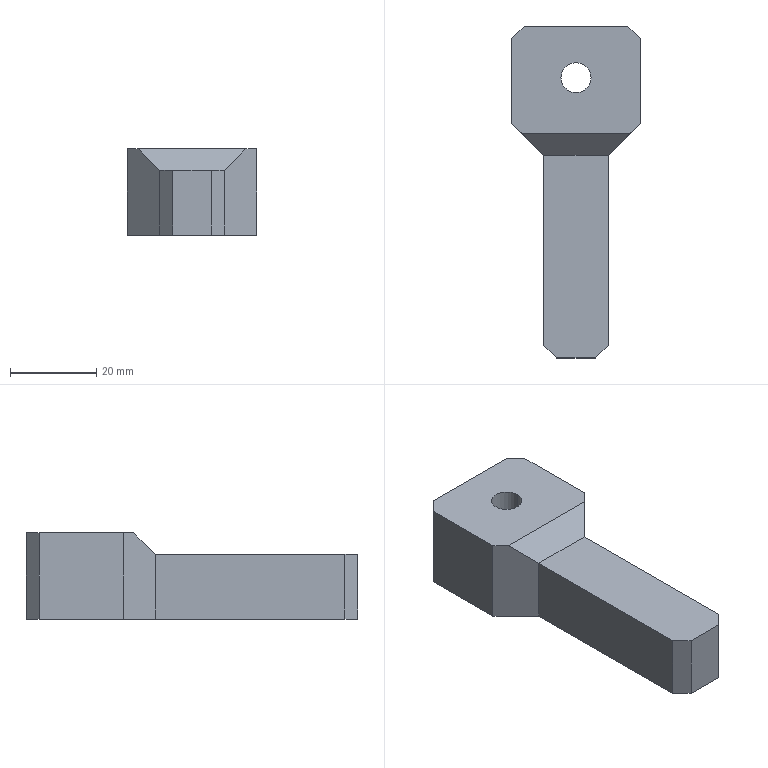Part | SolidWorks | features Chamfer 4, ICE 3, Cut 1, Extrusion 1 | 1 solid | 21 faces | box 30 x 77 x 20 mm | volume 24023 mm3 | plane 17 | cylinder 4 | commonest cylinder face diameters 7 x2 16 x2
STEP:
#1=CARTESIAN_POINT('',(-1.66,24.408,20.));
#2=VERTEX_POINT('',#1);
#3=CARTESIAN_POINT('',(-8.66,24.408,20.));
#4=VERTEX_POINT('',#3);
#5=CARTESIAN_POINT('',(-5.16,24.408,20.));
#6=DIRECTION('',(0.,0.,-1.));
#7=DIRECTION('',(-1.,0.,0.));
#8=AXIS2_PLACEMENT_3D('',#5,#6,#7);
#9=CIRCLE('',#8,3.5);
#10=EDGE_CURVE('',#2,#4,#9,.T.);
#11=ORIENTED_EDGE('',*,*,#10,.F.);
#12=CARTESIAN_POINT('',(-1.66,24.408,13.));
#13=VERTEX_POINT('',#12);
#14=CARTESIAN_POINT('',(-1.66,24.408,20.));
#15=DIRECTION('',(0.,0.,-1.));
#16=VECTOR('',#15,1000.);
#17=LINE('',#14,#16);
#18=EDGE_CURVE('',#2,#13,#17,.T.);
#19=ORIENTED_EDGE('',*,*,#18,.T.);
#20=CARTESIAN_POINT('',(-8.66,24.408,13.));
#21=VERTEX_POINT('',#20);
#22=CARTESIAN_POINT('',(-5.16,24.408,13.));
#23=DIRECTION('',(0.,0.,-1.));
#24=DIRECTION('',(-1.,0.,0.));
#25=AXIS2_PLACEMENT_3D('',#22,#23,#24);
#26=CIRCLE('',#25,3.5);
#27=EDGE_CURVE('',#13,#21,#26,.T.);
#28=ORIENTED_EDGE('',*,*,#27,.T.);
#29=CARTESIAN_POINT('',(-8.66,24.408,20.));
#30=DIRECTION('',(0.,0.,-1.));
#31=VECTOR('',#30,1000.);
#32=LINE('',#29,#31);
#33=EDGE_CURVE('',#4,#21,#32,.T.);
#34=ORIENTED_EDGE('',*,*,#33,.F.);
#35=EDGE_LOOP('',(#11,#19,#28,#34));
#36=FACE_OUTER_BOUND('',#35,.T.);
#37=CARTESIAN_POINT('',(-5.16,24.408,20.));
#38=DIRECTION('',(0.,0.,-1.));
#39=DIRECTION('',(-1.,0.,0.));
#40=AXIS2_PLACEMENT_3D('',#37,#38,#39);
#41=CYLINDRICAL_SURFACE('',#40,3.5);
#42=ADVANCED_FACE('',(#36),#41,.F.);
#43=CARTESIAN_POINT('',(2.84,24.408,13.));
#44=VERTEX_POINT('',#43);
#45=CARTESIAN_POINT('',(-13.16,24.408,13.));
#46=VERTEX_POINT('',#45);
#47=CARTESIAN_POINT('',(-5.16,24.408,13.));
#48=DIRECTION('',(0.,0.,-1.));
#49=DIRECTION('',(-1.,0.,0.));
#50=AXIS2_PLACEMENT_3D('',#47,#48,#49);
#51=CIRCLE('',#50,8.);
#52=EDGE_CURVE('',#44,#46,#51,.T.);
#53=ORIENTED_EDGE('',*,*,#52,.F.);
#54=CARTESIAN_POINT('',(2.84,24.408,0.));
#55=VERTEX_POINT('',#54);
#56=CARTESIAN_POINT('',(2.84,24.408,13.));
#57=DIRECTION('',(0.,0.,-1.));
#58=VECTOR('',#57,1000.);
#59=LINE('',#56,#58);
#60=EDGE_CURVE('',#44,#55,#59,.T.);
#61=ORIENTED_EDGE('',*,*,#60,.T.);
#62=CARTESIAN_POINT('',(-13.16,24.408,0.));
#63=VERTEX_POINT('',#62);
#64=CARTESIAN_POINT('',(-5.16,24.408,0.));
#65=DIRECTION('',(0.,0.,-1.));
#66=DIRECTION('',(-1.,0.,0.));
#67=AXIS2_PLACEMENT_3D('',#64,#65,#66);
#68=CIRCLE('',#67,8.);
#69=EDGE_CURVE('',#55,#63,#68,.T.);
#70=ORIENTED_EDGE('',*,*,#69,.T.);
#71=CARTESIAN_POINT('',(-13.16,24.408,13.));
#72=DIRECTION('',(0.,0.,-1.));
#73=VECTOR('',#72,1000.);
#74=LINE('',#71,#73);
#75=EDGE_CURVE('',#46,#63,#74,.T.);
#76=ORIENTED_EDGE('',*,*,#75,.F.);
#77=EDGE_LOOP('',(#53,#61,#70,#76));
#78=FACE_OUTER_BOUND('',#77,.T.);
#79=CARTESIAN_POINT('',(-5.16,24.408,13.));
#80=DIRECTION('',(0.,0.,-1.));
#81=DIRECTION('',(-1.,0.,0.));
#82=AXIS2_PLACEMENT_3D('',#79,#80,#81);
#83=CYLINDRICAL_SURFACE('',#82,8.);
#84=ADVANCED_FACE('',(#78),#83,.F.);
#85=CARTESIAN_POINT('',(-20.16,33.408,20.));
#86=VERTEX_POINT('',#85);
#87=CARTESIAN_POINT('',(-20.16,13.908,20.));
#88=VERTEX_POINT('',#87);
#89=CARTESIAN_POINT('',(-20.16,36.408,20.));
#90=DIRECTION('',(0.,-1.,0.));
#91=VECTOR('',#90,1000.);
#92=LINE('',#89,#91);
#93=EDGE_CURVE('',#86,#88,#92,.T.);
#94=ORIENTED_EDGE('',*,*,#93,.F.);
#95=CARTESIAN_POINT('',(-20.16,33.408,0.));
#96=VERTEX_POINT('',#95);
#97=CARTESIAN_POINT('',(-20.16,33.408,20.));
#98=DIRECTION('',(0.,0.,-1.));
#99=VECTOR('',#98,1000.);
#100=LINE('',#97,#99);
#101=EDGE_CURVE('',#86,#96,#100,.T.);
#102=ORIENTED_EDGE('',*,*,#101,.T.);
#103=CARTESIAN_POINT('',(-20.16,13.908,0.));
#104=VERTEX_POINT('',#103);
#105=CARTESIAN_POINT('',(-20.16,36.408,0.));
#106=DIRECTION('',(0.,-1.,0.));
#107=VECTOR('',#106,1000.);
#108=LINE('',#105,#107);
#109=EDGE_CURVE('',#96,#104,#108,.T.);
#110=ORIENTED_EDGE('',*,*,#109,.T.);
#111=CARTESIAN_POINT('',(-20.16,13.908,20.));
#112=DIRECTION('',(0.,0.,1.));
#113=VECTOR('',#112,1000.);
#114=LINE('',#111,#113);
#115=EDGE_CURVE('',#104,#88,#114,.T.);
#116=ORIENTED_EDGE('',*,*,#115,.T.);
#117=EDGE_LOOP('',(#94,#102,#110,#116));
#118=FACE_OUTER_BOUND('',#117,.T.);
#119=CARTESIAN_POINT('',(-20.16,36.408,20.));
#120=DIRECTION('',(1.,0.,0.));
#121=DIRECTION('',(0.,1.,0.));
#122=AXIS2_PLACEMENT_3D('',#119,#120,#121);
#123=PLANE('',#122);
#124=ADVANCED_FACE('',(#118),#123,.F.);
#125=CARTESIAN_POINT('',(-0.6603,-40.592,0.));
#126=VERTEX_POINT('',#125);
#127=CARTESIAN_POINT('',(-0.6603,-40.592,15.));
#128=VERTEX_POINT('',#127);
#129=CARTESIAN_POINT('',(-0.6603,-40.592,20.));
#130=DIRECTION('',(0.,0.,1.));
#131=VECTOR('',#130,1000.);
#132=LINE('',#129,#131);
#133=EDGE_CURVE('',#126,#128,#132,.T.);
#134=ORIENTED_EDGE('',*,*,#133,.T.);
#135=CARTESIAN_POINT('',(-9.66,-40.592,15.));
#136=VERTEX_POINT('',#135);
#137=CARTESIAN_POINT('',(-20.16,-40.592,15.));
#138=DIRECTION('',(-1.,0.,0.));
#139=VECTOR('',#138,1000.);
#140=LINE('',#137,#139);
#141=EDGE_CURVE('',#128,#136,#140,.T.);
#142=ORIENTED_EDGE('',*,*,#141,.T.);
#143=CARTESIAN_POINT('',(-9.66,-40.592,0.));
#144=VERTEX_POINT('',#143);
#145=CARTESIAN_POINT('',(-9.66,-40.592,20.));
#146=DIRECTION('',(0.,0.,-1.));
#147=VECTOR('',#146,1000.);
#148=LINE('',#145,#147);
#149=EDGE_CURVE('',#136,#144,#148,.T.);
#150=ORIENTED_EDGE('',*,*,#149,.T.);
#151=CARTESIAN_POINT('',(-20.16,-40.592,0.));
#152=DIRECTION('',(1.,0.,0.));
#153=VECTOR('',#152,1000.);
#154=LINE('',#151,#153);
#155=EDGE_CURVE('',#144,#126,#154,.T.);
#156=ORIENTED_EDGE('',*,*,#155,.T.);
#157=EDGE_LOOP('',(#134,#142,#150,#156));
#158=FACE_OUTER_BOUND('',#157,.T.);
#159=CARTESIAN_POINT('',(-20.16,-40.592,20.));
#160=DIRECTION('',(0.,1.,0.));
#161=DIRECTION('',(0.,0.,1.));
#162=AXIS2_PLACEMENT_3D('',#159,#160,#161);
#163=PLANE('',#162);
#164=ADVANCED_FACE('',(#158),#163,.F.);
#165=CARTESIAN_POINT('',(9.84,13.908,0.));
#166=VERTEX_POINT('',#165);
#167=CARTESIAN_POINT('',(9.84,33.408,0.));
#168=VERTEX_POINT('',#167);
#169=CARTESIAN_POINT('',(9.84,36.408,0.));
#170=DIRECTION('',(0.,1.,0.));
#171=VECTOR('',#170,1000.);
#172=LINE('',#169,#171);
#173=EDGE_CURVE('',#166,#168,#172,.T.);
#174=ORIENTED_EDGE('',*,*,#173,.T.);
#175=CARTESIAN_POINT('',(9.84,33.408,20.));
#176=VERTEX_POINT('',#175);
#177=CARTESIAN_POINT('',(9.84,33.408,20.));
#178=DIRECTION('',(0.,0.,1.));
#179=VECTOR('',#178,1000.);
#180=LINE('',#177,#179);
#181=EDGE_CURVE('',#168,#176,#180,.T.);
#182=ORIENTED_EDGE('',*,*,#181,.T.);
#183=CARTESIAN_POINT('',(9.84,13.908,20.));
#184=VERTEX_POINT('',#183);
#185=CARTESIAN_POINT('',(9.84,36.408,20.));
#186=DIRECTION('',(0.,1.,0.));
#187=VECTOR('',#186,1000.);
#188=LINE('',#185,#187);
#189=EDGE_CURVE('',#184,#176,#188,.T.);
#190=ORIENTED_EDGE('',*,*,#189,.F.);
#191=CARTESIAN_POINT('',(9.84,13.908,20.));
#192=DIRECTION('',(0.,0.,-1.));
#193=VECTOR('',#192,1000.);
#194=LINE('',#191,#193);
#195=EDGE_CURVE('',#184,#166,#194,.T.);
#196=ORIENTED_EDGE('',*,*,#195,.T.);
#197=EDGE_LOOP('',(#174,#182,#190,#196));
#198=FACE_OUTER_BOUND('',#197,.T.);
#199=CARTESIAN_POINT('',(9.84,36.408,20.));
#200=DIRECTION('',(-1.,0.,0.));
#201=DIRECTION('',(0.,-1.,0.));
#202=AXIS2_PLACEMENT_3D('',#199,#200,#201);
#203=PLANE('',#202);
#204=ADVANCED_FACE('',(#198),#203,.F.);
#205=CARTESIAN_POINT('',(6.84,36.408,20.));
#206=VERTEX_POINT('',#205);
#207=CARTESIAN_POINT('',(-17.16,36.408,20.));
#208=VERTEX_POINT('',#207);
#209=CARTESIAN_POINT('',(-20.16,36.408,20.));
#210=DIRECTION('',(-1.,0.,0.));
#211=VECTOR('',#210,1000.);
#212=LINE('',#209,#211);
#213=EDGE_CURVE('',#206,#208,#212,.T.);
#214=ORIENTED_EDGE('',*,*,#213,.F.);
#215=CARTESIAN_POINT('',(6.84,36.408,0.));
#216=VERTEX_POINT('',#215);
#217=CARTESIAN_POINT('',(6.84,36.408,20.));
#218=DIRECTION('',(0.,0.,-1.));
#219=VECTOR('',#218,1000.);
#220=LINE('',#217,#219);
#221=EDGE_CURVE('',#206,#216,#220,.T.);
#222=ORIENTED_EDGE('',*,*,#221,.T.);
#223=CARTESIAN_POINT('',(-17.16,36.408,0.));
#224=VERTEX_POINT('',#223);
#225=CARTESIAN_POINT('',(-20.16,36.408,0.));
#226=DIRECTION('',(-1.,0.,0.));
#227=VECTOR('',#226,1000.);
#228=LINE('',#225,#227);
#229=EDGE_CURVE('',#216,#224,#228,.T.);
#230=ORIENTED_EDGE('',*,*,#229,.T.);
#231=CARTESIAN_POINT('',(-17.16,36.408,20.));
#232=DIRECTION('',(0.,0.,1.));
#233=VECTOR('',#232,1000.);
#234=LINE('',#231,#233);
#235=EDGE_CURVE('',#224,#208,#234,.T.);
#236=ORIENTED_EDGE('',*,*,#235,.T.);
#237=EDGE_LOOP('',(#214,#222,#230,#236));
#238=FACE_OUTER_BOUND('',#237,.T.);
#239=CARTESIAN_POINT('',(-20.16,36.408,20.));
#240=DIRECTION('',(0.,-1.,0.));
#241=DIRECTION('',(0.,0.,-1.));
#242=AXIS2_PLACEMENT_3D('',#239,#240,#241);
#243=PLANE('',#242);
#244=ADVANCED_FACE('',(#238),#243,.F.);
#245=CARTESIAN_POINT('',(-17.66,11.408,20.));
#246=VERTEX_POINT('',#245);
#247=CARTESIAN_POINT('',(-3.126,-3.126,20.));
#248=DIRECTION('',(0.7071,-0.7071,0.));
#249=VECTOR('',#248,1000.);
#250=LINE('',#247,#249);
#251=EDGE_CURVE('',#88,#246,#250,.T.);
#252=ORIENTED_EDGE('',*,*,#251,.T.);
#253=CARTESIAN_POINT('',(7.34,11.408,20.));
#254=VERTEX_POINT('',#253);
#255=CARTESIAN_POINT('',(2.34,11.408,20.));
#256=DIRECTION('',(1.,0.,0.));
#257=VECTOR('',#256,1000.);
#258=LINE('',#255,#257);
#259=EDGE_CURVE('',#246,#254,#258,.T.);
#260=ORIENTED_EDGE('',*,*,#259,.T.);
#261=CARTESIAN_POINT('',(-2.034,2.034,20.));
#262=DIRECTION('',(0.7071,0.7071,0.));
#263=VECTOR('',#262,1000.);
#264=LINE('',#261,#263);
#265=EDGE_CURVE('',#254,#184,#264,.T.);
#266=ORIENTED_EDGE('',*,*,#265,.T.);
#267=ORIENTED_EDGE('',*,*,#189,.T.);
#268=CARTESIAN_POINT('',(21.624,21.624,20.));
#269=DIRECTION('',(-0.7071,0.7071,0.));
#270=VECTOR('',#269,1000.);
#271=LINE('',#268,#270);
#272=EDGE_CURVE('',#176,#206,#271,.T.);
#273=ORIENTED_EDGE('',*,*,#272,.T.);
#274=ORIENTED_EDGE('',*,*,#213,.T.);
#275=CARTESIAN_POINT('',(-26.784,26.784,20.));
#276=DIRECTION('',(-0.7071,-0.7071,0.));
#277=VECTOR('',#276,1000.);
#278=LINE('',#275,#277);
#279=EDGE_CURVE('',#208,#86,#278,.T.);
#280=ORIENTED_EDGE('',*,*,#279,.T.);
#281=ORIENTED_EDGE('',*,*,#93,.T.);
#282=EDGE_LOOP('',(#252,#260,#266,#267,#273,#274,#280,#281));
#283=FACE_OUTER_BOUND('',#282,.T.);
#284=CARTESIAN_POINT('',(-5.16,24.408,20.));
#285=DIRECTION('',(0.,0.,-1.));
#286=DIRECTION('',(-1.,0.,0.));
#287=AXIS2_PLACEMENT_3D('',#284,#285,#286);
#288=CIRCLE('',#287,3.5);
#289=EDGE_CURVE('',#4,#2,#288,.T.);
#290=ORIENTED_EDGE('',*,*,#289,.T.);
#291=ORIENTED_EDGE('',*,*,#10,.T.);
#292=EDGE_LOOP('',(#290,#291));
#293=FACE_BOUND('',#292,.T.);
#294=CARTESIAN_POINT('',(0.,0.,20.));
#295=DIRECTION('',(0.,0.,1.));
#296=DIRECTION('',(1.,0.,0.));
#297=AXIS2_PLACEMENT_3D('',#294,#295,#296);
#298=PLANE('',#297);
#299=ADVANCED_FACE('',(#283,#293),#298,.T.);
#300=CARTESIAN_POINT('',(-5.16,24.408,0.));
#301=DIRECTION('',(0.,0.,-1.));
#302=DIRECTION('',(-1.,0.,0.));
#303=AXIS2_PLACEMENT_3D('',#300,#301,#302);
#304=CIRCLE('',#303,8.);
#305=EDGE_CURVE('',#63,#55,#304,.T.);
#306=ORIENTED_EDGE('',*,*,#305,.F.);
#307=ORIENTED_EDGE('',*,*,#69,.F.);
#308=EDGE_LOOP('',(#306,#307));
#309=FACE_BOUND('',#308,.T.);
#310=ORIENTED_EDGE('',*,*,#229,.F.);
#311=CARTESIAN_POINT('',(6.84,36.408,0.));
#312=DIRECTION('',(0.7071,-0.7071,0.));
#313=VECTOR('',#312,1000.);
#314=LINE('',#311,#313);
#315=EDGE_CURVE('',#216,#168,#314,.T.);
#316=ORIENTED_EDGE('',*,*,#315,.T.);
#317=ORIENTED_EDGE('',*,*,#173,.F.);
#318=CARTESIAN_POINT('',(2.34,6.408,0.));
#319=VERTEX_POINT('',#318);
#320=CARTESIAN_POINT('',(9.84,13.908,0.));
#321=DIRECTION('',(-0.7071,-0.7071,0.));
#322=VECTOR('',#321,1000.);
#323=LINE('',#320,#322);
#324=EDGE_CURVE('',#166,#319,#323,.T.);
#325=ORIENTED_EDGE('',*,*,#324,.T.);
#326=CARTESIAN_POINT('',(2.34,-37.592,0.));
#327=VERTEX_POINT('',#326);
#328=CARTESIAN_POINT('',(2.34,6.408,0.));
#329=DIRECTION('',(0.,-1.,0.));
#330=VECTOR('',#329,1000.);
#331=LINE('',#328,#330);
#332=EDGE_CURVE('',#319,#327,#331,.T.);
#333=ORIENTED_EDGE('',*,*,#332,.T.);
#334=CARTESIAN_POINT('',(-0.6603,-40.592,0.));
#335=DIRECTION('',(-0.7071,-0.7071,0.));
#336=VECTOR('',#335,1000.);
#337=LINE('',#334,#336);
#338=EDGE_CURVE('',#327,#126,#337,.T.);
#339=ORIENTED_EDGE('',*,*,#338,.T.);
#340=ORIENTED_EDGE('',*,*,#155,.F.);
#341=CARTESIAN_POINT('',(-12.66,-37.592,0.));
#342=VERTEX_POINT('',#341);
#343=CARTESIAN_POINT('',(-9.66,-40.592,0.));
#344=DIRECTION('',(-0.7071,0.7071,0.));
#345=VECTOR('',#344,1000.);
#346=LINE('',#343,#345);
#347=EDGE_CURVE('',#144,#342,#346,.T.);
#348=ORIENTED_EDGE('',*,*,#347,.T.);
#349=CARTESIAN_POINT('',(-12.66,6.408,0.));
#350=VERTEX_POINT('',#349);
#351=CARTESIAN_POINT('',(-12.66,0.,0.));
#352=DIRECTION('',(0.,1.,0.));
#353=VECTOR('',#352,1000.);
#354=LINE('',#351,#353);
#355=EDGE_CURVE('',#342,#350,#354,.T.);
#356=ORIENTED_EDGE('',*,*,#355,.T.);
#357=CARTESIAN_POINT('',(-20.16,13.908,0.));
#358=DIRECTION('',(-0.7071,0.7071,0.));
#359=VECTOR('',#358,1000.);
#360=LINE('',#357,#359);
#361=EDGE_CURVE('',#350,#104,#360,.T.);
#362=ORIENTED_EDGE('',*,*,#361,.T.);
#363=ORIENTED_EDGE('',*,*,#109,.F.);
#364=CARTESIAN_POINT('',(-20.16,33.408,0.));
#365=DIRECTION('',(0.7071,0.7071,0.));
#366=VECTOR('',#365,1000.);
#367=LINE('',#364,#366);
#368=EDGE_CURVE('',#96,#224,#367,.T.);
#369=ORIENTED_EDGE('',*,*,#368,.T.);
#370=EDGE_LOOP('',(#310,#316,#317,#325,#333,#339,#340,#348,#356,#362,#363,#369));
#371=FACE_OUTER_BOUND('',#370,.T.);
#372=CARTESIAN_POINT('',(0.,0.,0.));
#373=DIRECTION('',(0.,0.,1.));
#374=DIRECTION('',(1.,0.,0.));
#375=AXIS2_PLACEMENT_3D('',#372,#373,#374);
#376=PLANE('',#375);
#377=ADVANCED_FACE('',(#309,#371),#376,.F.);
#378=ORIENTED_EDGE('',*,*,#60,.F.);
#379=CARTESIAN_POINT('',(-5.16,24.408,13.));
#380=DIRECTION('',(0.,0.,-1.));
#381=DIRECTION('',(-1.,0.,0.));
#382=AXIS2_PLACEMENT_3D('',#379,#380,#381);
#383=CIRCLE('',#382,8.);
#384=EDGE_CURVE('',#46,#44,#383,.T.);
#385=ORIENTED_EDGE('',*,*,#384,.F.);
#386=ORIENTED_EDGE('',*,*,#75,.T.);
#387=ORIENTED_EDGE('',*,*,#305,.T.);
#388=EDGE_LOOP('',(#378,#385,#386,#387));
#389=FACE_OUTER_BOUND('',#388,.T.);
#390=CARTESIAN_POINT('',(-5.16,24.408,13.));
#391=DIRECTION('',(0.,0.,-1.));
#392=DIRECTION('',(-1.,0.,0.));
#393=AXIS2_PLACEMENT_3D('',#390,#391,#392);
#394=CYLINDRICAL_SURFACE('',#393,8.);
#395=ADVANCED_FACE('',(#389),#394,.F.);
#396=CARTESIAN_POINT('',(-5.16,24.408,13.));
#397=DIRECTION('',(0.,0.,-1.));
#398=DIRECTION('',(-1.,0.,0.));
#399=AXIS2_PLACEMENT_3D('',#396,#397,#398);
#400=CIRCLE('',#399,3.5);
#401=EDGE_CURVE('',#21,#13,#400,.T.);
#402=ORIENTED_EDGE('',*,*,#401,.F.);
#403=ORIENTED_EDGE('',*,*,#27,.F.);
#404=EDGE_LOOP('',(#402,#403));
#405=FACE_BOUND('',#404,.T.);
#406=ORIENTED_EDGE('',*,*,#384,.T.);
#407=ORIENTED_EDGE('',*,*,#52,.T.);
#408=EDGE_LOOP('',(#406,#407));
#409=FACE_OUTER_BOUND('',#408,.T.);
#410=CARTESIAN_POINT('',(-5.16,24.408,13.));
#411=DIRECTION('',(0.,0.,-1.));
#412=DIRECTION('',(-1.,0.,0.));
#413=AXIS2_PLACEMENT_3D('',#410,#411,#412);
#414=PLANE('',#413);
#415=ADVANCED_FACE('',(#405,#409),#414,.T.);
#416=ORIENTED_EDGE('',*,*,#18,.F.);
#417=ORIENTED_EDGE('',*,*,#289,.F.);
#418=ORIENTED_EDGE('',*,*,#33,.T.);
#419=ORIENTED_EDGE('',*,*,#401,.T.);
#420=EDGE_LOOP('',(#416,#417,#418,#419));
#421=FACE_OUTER_BOUND('',#420,.T.);
#422=CARTESIAN_POINT('',(-5.16,24.408,20.));
#423=DIRECTION('',(0.,0.,-1.));
#424=DIRECTION('',(-1.,0.,0.));
#425=AXIS2_PLACEMENT_3D('',#422,#423,#424);
#426=CYLINDRICAL_SURFACE('',#425,3.5);
#427=ADVANCED_FACE('',(#421),#426,.F.);
#428=CARTESIAN_POINT('',(2.34,6.408,15.));
#429=VERTEX_POINT('',#428);
#430=CARTESIAN_POINT('',(2.34,6.408,0.));
#431=DIRECTION('',(0.,0.,1.));
#432=VECTOR('',#431,1000.);
#433=LINE('',#430,#432);
#434=EDGE_CURVE('',#319,#429,#433,.T.);
#435=ORIENTED_EDGE('',*,*,#434,.T.);
#436=CARTESIAN_POINT('',(2.34,-37.592,15.));
#437=VERTEX_POINT('',#436);
#438=CARTESIAN_POINT('',(2.34,6.408,15.));
#439=DIRECTION('',(0.,-1.,0.));
#440=VECTOR('',#439,1000.);
#441=LINE('',#438,#440);
#442=EDGE_CURVE('',#429,#437,#441,.T.);
#443=ORIENTED_EDGE('',*,*,#442,.T.);
#444=CARTESIAN_POINT('',(2.34,-37.592,0.));
#445=DIRECTION('',(0.,0.,-1.));
#446=VECTOR('',#445,1000.);
#447=LINE('',#444,#446);
#448=EDGE_CURVE('',#437,#327,#447,.T.);
#449=ORIENTED_EDGE('',*,*,#448,.T.);
#450=ORIENTED_EDGE('',*,*,#332,.F.);
#451=EDGE_LOOP('',(#435,#443,#449,#450));
#452=FACE_OUTER_BOUND('',#451,.T.);
#453=CARTESIAN_POINT('',(2.34,6.408,0.));
#454=DIRECTION('',(-1.,0.,0.));
#455=DIRECTION('',(0.,-1.,0.));
#456=AXIS2_PLACEMENT_3D('',#453,#454,#455);
#457=PLANE('',#456);
#458=ADVANCED_FACE('',(#452),#457,.F.);
#459=CARTESIAN_POINT('',(-12.66,-37.592,15.));
#460=VERTEX_POINT('',#459);
#461=CARTESIAN_POINT('',(-12.66,-37.592,0.));
#462=DIRECTION('',(0.,0.,1.));
#463=VECTOR('',#462,1000.);
#464=LINE('',#461,#463);
#465=EDGE_CURVE('',#342,#460,#464,.T.);
#466=ORIENTED_EDGE('',*,*,#465,.T.);
#467=CARTESIAN_POINT('',(-12.66,6.408,15.));
#468=VERTEX_POINT('',#467);
#469=CARTESIAN_POINT('',(-12.66,6.408,15.));
#470=DIRECTION('',(0.,1.,0.));
#471=VECTOR('',#470,1000.);
#472=LINE('',#469,#471);
#473=EDGE_CURVE('',#460,#468,#472,.T.);
#474=ORIENTED_EDGE('',*,*,#473,.T.);
#475=CARTESIAN_POINT('',(-12.66,6.408,0.));
#476=DIRECTION('',(0.,0.,1.));
#477=VECTOR('',#476,1000.);
#478=LINE('',#475,#477);
#479=EDGE_CURVE('',#350,#468,#478,.T.);
#480=ORIENTED_EDGE('',*,*,#479,.F.);
#481=ORIENTED_EDGE('',*,*,#355,.F.);
#482=EDGE_LOOP('',(#466,#474,#480,#481));
#483=FACE_OUTER_BOUND('',#482,.T.);
#484=CARTESIAN_POINT('',(-12.66,6.408,0.));
#485=DIRECTION('',(1.,0.,0.));
#486=DIRECTION('',(0.,1.,0.));
#487=AXIS2_PLACEMENT_3D('',#484,#485,#486);
#488=PLANE('',#487);
#489=ADVANCED_FACE('',(#483),#488,.F.);
#490=CARTESIAN_POINT('',(-0.6603,-40.592,15.));
#491=DIRECTION('',(0.7071,0.7071,0.));
#492=VECTOR('',#491,1000.);
#493=LINE('',#490,#492);
#494=EDGE_CURVE('',#128,#437,#493,.T.);
#495=ORIENTED_EDGE('',*,*,#494,.F.);
#496=ORIENTED_EDGE('',*,*,#133,.F.);
#497=ORIENTED_EDGE('',*,*,#338,.F.);
#498=ORIENTED_EDGE('',*,*,#448,.F.);
#499=EDGE_LOOP('',(#495,#496,#497,#498));
#500=FACE_OUTER_BOUND('',#499,.T.);
#501=CARTESIAN_POINT('',(-0.6603,-40.592,20.));
#502=DIRECTION('',(-0.7071,0.7071,0.));
#503=DIRECTION('',(0.,0.,1.));
#504=AXIS2_PLACEMENT_3D('',#501,#502,#503);
#505=PLANE('',#504);
#506=ADVANCED_FACE('',(#500),#505,.F.);
#507=CARTESIAN_POINT('',(-9.66,-40.592,15.));
#508=DIRECTION('',(0.7071,-0.7071,0.));
#509=VECTOR('',#508,1000.);
#510=LINE('',#507,#509);
#511=EDGE_CURVE('',#460,#136,#510,.T.);
#512=ORIENTED_EDGE('',*,*,#511,.F.);
#513=ORIENTED_EDGE('',*,*,#465,.F.);
#514=ORIENTED_EDGE('',*,*,#347,.F.);
#515=ORIENTED_EDGE('',*,*,#149,.F.);
#516=EDGE_LOOP('',(#512,#513,#514,#515));
#517=FACE_OUTER_BOUND('',#516,.T.);
#518=CARTESIAN_POINT('',(-9.66,-40.592,20.));
#519=DIRECTION('',(0.7071,0.7071,0.));
#520=DIRECTION('',(0.,0.,-1.));
#521=AXIS2_PLACEMENT_3D('',#518,#519,#520);
#522=PLANE('',#521);
#523=ADVANCED_FACE('',(#517),#522,.F.);
#524=ORIENTED_EDGE('',*,*,#265,.F.);
#525=CARTESIAN_POINT('',(9.006,13.074,21.667));
#526=DIRECTION('',(-0.5774,-0.5774,-0.5774));
#527=VECTOR('',#526,1000.);
#528=LINE('',#525,#527);
#529=EDGE_CURVE('',#254,#429,#528,.T.);
#530=ORIENTED_EDGE('',*,*,#529,.T.);
#531=ORIENTED_EDGE('',*,*,#434,.F.);
#532=ORIENTED_EDGE('',*,*,#324,.F.);
#533=ORIENTED_EDGE('',*,*,#195,.F.);
#534=EDGE_LOOP('',(#524,#530,#531,#532,#533));
#535=FACE_OUTER_BOUND('',#534,.T.);
#536=CARTESIAN_POINT('',(9.84,13.908,20.));
#537=DIRECTION('',(-0.7071,0.7071,0.));
#538=DIRECTION('',(0.,0.,-1.));
#539=AXIS2_PLACEMENT_3D('',#536,#537,#538);
#540=PLANE('',#539);
#541=ADVANCED_FACE('',(#535),#540,.F.);
#542=ORIENTED_EDGE('',*,*,#479,.T.);
#543=CARTESIAN_POINT('',(-19.327,13.074,21.667));
#544=DIRECTION('',(-0.5774,0.5774,0.5774));
#545=VECTOR('',#544,1000.);
#546=LINE('',#543,#545);
#547=EDGE_CURVE('',#468,#246,#546,.T.);
#548=ORIENTED_EDGE('',*,*,#547,.T.);
#549=ORIENTED_EDGE('',*,*,#251,.F.);
#550=ORIENTED_EDGE('',*,*,#115,.F.);
#551=ORIENTED_EDGE('',*,*,#361,.F.);
#552=EDGE_LOOP('',(#542,#548,#549,#550,#551));
#553=FACE_OUTER_BOUND('',#552,.T.);
#554=CARTESIAN_POINT('',(-20.16,13.908,20.));
#555=DIRECTION('',(0.7071,0.7071,0.));
#556=DIRECTION('',(0.,0.,1.));
#557=AXIS2_PLACEMENT_3D('',#554,#555,#556);
#558=PLANE('',#557);
#559=ADVANCED_FACE('',(#553),#558,.F.);
#560=ORIENTED_EDGE('',*,*,#272,.F.);
#561=ORIENTED_EDGE('',*,*,#181,.F.);
#562=ORIENTED_EDGE('',*,*,#315,.F.);
#563=ORIENTED_EDGE('',*,*,#221,.F.);
#564=EDGE_LOOP('',(#560,#561,#562,#563));
#565=FACE_OUTER_BOUND('',#564,.T.);
#566=CARTESIAN_POINT('',(6.84,36.408,20.));
#567=DIRECTION('',(-0.7071,-0.7071,0.));
#568=DIRECTION('',(0.,0.,-1.));
#569=AXIS2_PLACEMENT_3D('',#566,#567,#568);
#570=PLANE('',#569);
#571=ADVANCED_FACE('',(#565),#570,.F.);
#572=ORIENTED_EDGE('',*,*,#279,.F.);
#573=ORIENTED_EDGE('',*,*,#235,.F.);
#574=ORIENTED_EDGE('',*,*,#368,.F.);
#575=ORIENTED_EDGE('',*,*,#101,.F.);
#576=EDGE_LOOP('',(#572,#573,#574,#575));
#577=FACE_OUTER_BOUND('',#576,.T.);
#578=CARTESIAN_POINT('',(-20.16,33.408,20.));
#579=DIRECTION('',(0.7071,-0.7071,0.));
#580=DIRECTION('',(0.,0.,-1.));
#581=AXIS2_PLACEMENT_3D('',#578,#579,#580);
#582=PLANE('',#581);
#583=ADVANCED_FACE('',(#577),#582,.F.);
#584=CARTESIAN_POINT('',(9.84,6.408,15.));
#585=DIRECTION('',(-1.,0.,0.));
#586=VECTOR('',#585,1000.);
#587=LINE('',#584,#586);
#588=EDGE_CURVE('',#429,#468,#587,.T.);
#589=ORIENTED_EDGE('',*,*,#588,.T.);
#590=ORIENTED_EDGE('',*,*,#473,.F.);
#591=ORIENTED_EDGE('',*,*,#511,.T.);
#592=ORIENTED_EDGE('',*,*,#141,.F.);
#593=ORIENTED_EDGE('',*,*,#494,.T.);
#594=ORIENTED_EDGE('',*,*,#442,.F.);
#595=EDGE_LOOP('',(#589,#590,#591,#592,#593,#594));
#596=FACE_OUTER_BOUND('',#595,.T.);
#597=CARTESIAN_POINT('',(9.84,6.408,15.));
#598=DIRECTION('',(0.,0.,-1.));
#599=DIRECTION('',(0.,1.,0.));
#600=AXIS2_PLACEMENT_3D('',#597,#598,#599);
#601=PLANE('',#600);
#602=ADVANCED_FACE('',(#596),#601,.F.);
#603=ORIENTED_EDGE('',*,*,#529,.F.);
#604=ORIENTED_EDGE('',*,*,#259,.F.);
#605=ORIENTED_EDGE('',*,*,#547,.F.);
#606=ORIENTED_EDGE('',*,*,#588,.F.);
#607=EDGE_LOOP('',(#603,#604,#605,#606));
#608=FACE_OUTER_BOUND('',#607,.T.);
#609=CARTESIAN_POINT('',(9.84,6.408,15.));
#610=DIRECTION('',(0.,-0.7071,0.7071));
#611=DIRECTION('',(1.,0.,0.));
#612=AXIS2_PLACEMENT_3D('',#609,#610,#611);
#613=PLANE('',#612);
#614=ADVANCED_FACE('',(#608),#613,.T.);
#615=CLOSED_SHELL('',(#42,#84,#124,#164,#204,#244,#299,#377,#395,#415,#427,#458,#489,#506,#523,#541,#559,#571,#583,#602,#614));
#616=MANIFOLD_SOLID_BREP('',#615);
#617=CARTESIAN_POINT('',(0.,0.,0.));
#618=DIRECTION('',(0.,0.,1.));
#619=DIRECTION('',(1.,0.,0.));
#620=AXIS2_PLACEMENT_3D('',#617,#618,#619);
#621=(LENGTH_UNIT()NAMED_UNIT(*)SI_UNIT(.MILLI.,.METRE.));
#622=UNCERTAINTY_MEASURE_WITH_UNIT(LENGTH_MEASURE(0.00001),#621,'','');
#623=(NAMED_UNIT(*)PLANE_ANGLE_UNIT()SI_UNIT($,.RADIAN.));
#624=(NAMED_UNIT(*)SI_UNIT($,.STERADIAN.)SOLID_ANGLE_UNIT());
#625=(GEOMETRIC_REPRESENTATION_CONTEXT(3)GLOBAL_UNCERTAINTY_ASSIGNED_CONTEXT((#622))GLOBAL_UNIT_ASSIGNED_CONTEXT((#621,#623,#624))REPRESENTATION_CONTEXT('',''));
#626=ADVANCED_BREP_SHAPE_REPRESENTATION('',(#616,#620),#625);